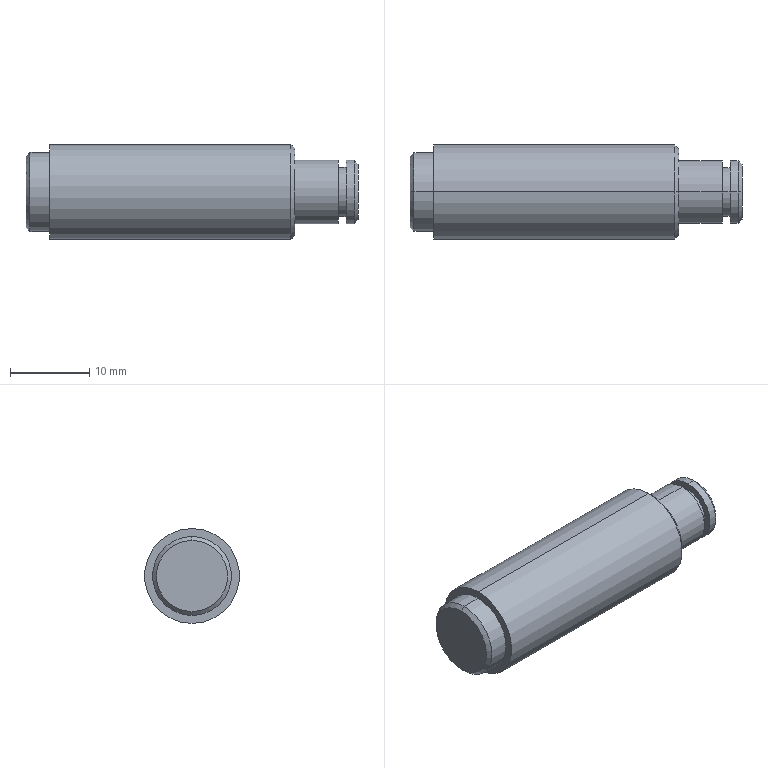Part | STEP file | 1 solid | 22 faces | box 42 x 12 x 12 mm | volume 4112 mm3 | cylinder 10 | cone 6 | plane 6 | commonest cylinder face diameters 8 x4 6.2 x2 10 x2 12 x2
STEP:
#1=CARTESIAN_POINT('',(0.,0.,0.));
#2=DIRECTION('',(0.,0.,1.));
#3=DIRECTION('',(1.,0.,0.));
#4=AXIS2_PLACEMENT_3D('',#1,#2,#3);
#5=CARTESIAN_POINT('',(3.,0.,-6.));
#6=VERTEX_POINT('',#5);
#7=CARTESIAN_POINT('',(3.,0.,6.));
#8=VERTEX_POINT('',#7);
#9=CARTESIAN_POINT('',(3.,0.,0.));
#10=DIRECTION('',(1.,0.,0.));
#11=DIRECTION('',(0.,0.,-1.));
#12=AXIS2_PLACEMENT_3D('',#9,#10,#11);
#13=CIRCLE('',#12,6.);
#14=CARTESIAN_POINT('',(18.5,0.,0.));
#15=DIRECTION('',(1.,0.,0.));
#16=DIRECTION('',(0.,0.,-1.));
#17=AXIS2_PLACEMENT_3D('',#14,#15,#16);
#18=CYLINDRICAL_SURFACE('',#17,6.);
#19=CARTESIAN_POINT('',(0.,-15.5));
#20=DIRECTION('',(1.,0.));
#21=VECTOR('',#20,1.);
#22=LINE('',#19,#21);
#23=(GEOMETRIC_REPRESENTATION_CONTEXT(2)PARAMETRIC_REPRESENTATION_CONTEXT()REPRESENTATION_CONTEXT('',''));
#24=DEFINITIONAL_REPRESENTATION('',(#22),#23);
#25=PCURVE('',#18,#24);
#26=CARTESIAN_POINT('',(3.,5.5,0.));
#27=DIRECTION('',(-1.,0.,0.));
#28=DIRECTION('',(0.,0.,1.));
#29=AXIS2_PLACEMENT_3D('',#26,#27,#28);
#30=PLANE('',#29);
#31=CARTESIAN_POINT('',(-6.,-5.5));
#32=CARTESIAN_POINT('',(-6.,4.892));
#33=CARTESIAN_POINT('',(3.,-0.3038));
#34=CARTESIAN_POINT('',(12.,-5.5));
#35=CARTESIAN_POINT('',(3.,-10.696));
#36=CARTESIAN_POINT('',(-6.,-15.892));
#37=CARTESIAN_POINT('',(-6.,-5.5));
#38=(BOUNDED_CURVE()B_SPLINE_CURVE(2,(#31,#32,#33,#34,#35,#36,#37),.UNSPECIFIED.,.T.,.F.)B_SPLINE_CURVE_WITH_KNOTS((1,2,2,2,2,1),(-2.094,0.,2.094,4.189,6.283,8.378),.UNSPECIFIED.)CURVE()GEOMETRIC_REPRESENTATION_ITEM()RATIONAL_B_SPLINE_CURVE((1.,0.5,1.,0.5,1.,0.5,1.))REPRESENTATION_ITEM(''));
#39=(GEOMETRIC_REPRESENTATION_CONTEXT(2)PARAMETRIC_REPRESENTATION_CONTEXT()REPRESENTATION_CONTEXT('',''));
#40=DEFINITIONAL_REPRESENTATION('',(#38),#39);
#41=PCURVE('',#30,#40);
#42=SURFACE_CURVE('',#13,(#25,#41),.PCURVE_S1.);
#43=EDGE_CURVE('',#6,#8,#42,.T.);
#44=ORIENTED_EDGE('',*,*,#43,.T.);
#45=CARTESIAN_POINT('',(33.5,0.,6.));
#46=VERTEX_POINT('',#45);
#47=CARTESIAN_POINT('',(18.5,0.,6.));
#48=DIRECTION('',(1.,0.,0.));
#49=VECTOR('',#48,1.);
#50=LINE('',#47,#49);
#51=CARTESIAN_POINT('',(3.142,0.));
#52=DIRECTION('',(0.,1.));
#53=VECTOR('',#52,1.);
#54=LINE('',#51,#53);
#55=(GEOMETRIC_REPRESENTATION_CONTEXT(2)PARAMETRIC_REPRESENTATION_CONTEXT()REPRESENTATION_CONTEXT('',''));
#56=DEFINITIONAL_REPRESENTATION('',(#54),#55);
#57=PCURVE('',#18,#56);
#58=CARTESIAN_POINT('',(18.5,0.,0.));
#59=DIRECTION('',(1.,0.,0.));
#60=DIRECTION('',(0.,0.,-1.));
#61=AXIS2_PLACEMENT_3D('',#58,#59,#60);
#62=CYLINDRICAL_SURFACE('',#61,6.);
#63=CARTESIAN_POINT('',(3.142,0.));
#64=DIRECTION('',(0.,1.));
#65=VECTOR('',#64,1.);
#66=LINE('',#63,#65);
#67=(GEOMETRIC_REPRESENTATION_CONTEXT(2)PARAMETRIC_REPRESENTATION_CONTEXT()REPRESENTATION_CONTEXT('',''));
#68=DEFINITIONAL_REPRESENTATION('',(#66),#67);
#69=PCURVE('',#62,#68);
#70=SURFACE_CURVE('',#50,(#57,#69),.PCURVE_S1.);
#71=EDGE_CURVE('',#8,#46,#70,.T.);
#72=ORIENTED_EDGE('',*,*,#71,.T.);
#73=CARTESIAN_POINT('',(33.5,0.,-6.));
#74=VERTEX_POINT('',#73);
#75=CARTESIAN_POINT('',(33.5,0.,0.));
#76=DIRECTION('',(-1.,0.,0.));
#77=DIRECTION('',(0.,0.,-1.));
#78=AXIS2_PLACEMENT_3D('',#75,#76,#77);
#79=CIRCLE('',#78,6.);
#80=CARTESIAN_POINT('',(6.283,15.));
#81=DIRECTION('',(-1.,0.));
#82=VECTOR('',#81,1.);
#83=LINE('',#80,#82);
#84=(GEOMETRIC_REPRESENTATION_CONTEXT(2)PARAMETRIC_REPRESENTATION_CONTEXT()REPRESENTATION_CONTEXT('',''));
#85=DEFINITIONAL_REPRESENTATION('',(#83),#84);
#86=PCURVE('',#18,#85);
#87=CARTESIAN_POINT('',(33.5,0.,0.));
#88=DIRECTION('',(-1.,0.,0.));
#89=DIRECTION('',(0.,0.,1.));
#90=AXIS2_PLACEMENT_3D('',#87,#88,#89);
#91=CONICAL_SURFACE('',#90,6.,0.7854);
#92=CARTESIAN_POINT('',(-3.142,0.));
#93=DIRECTION('',(1.,0.));
#94=VECTOR('',#93,1.);
#95=LINE('',#92,#94);
#96=(GEOMETRIC_REPRESENTATION_CONTEXT(2)PARAMETRIC_REPRESENTATION_CONTEXT()REPRESENTATION_CONTEXT('',''));
#97=DEFINITIONAL_REPRESENTATION('',(#95),#96);
#98=PCURVE('',#91,#97);
#99=SURFACE_CURVE('',#79,(#86,#98),.PCURVE_S1.);
#100=EDGE_CURVE('',#46,#74,#99,.T.);
#101=ORIENTED_EDGE('',*,*,#100,.T.);
#102=CARTESIAN_POINT('',(18.5,0.,-6.));
#103=DIRECTION('',(1.,0.,0.));
#104=VECTOR('',#103,1.);
#105=LINE('',#102,#104);
#106=CARTESIAN_POINT('',(0.,0.));
#107=DIRECTION('',(0.,1.));
#108=VECTOR('',#107,1.);
#109=LINE('',#106,#108);
#110=(GEOMETRIC_REPRESENTATION_CONTEXT(2)PARAMETRIC_REPRESENTATION_CONTEXT()REPRESENTATION_CONTEXT('',''));
#111=DEFINITIONAL_REPRESENTATION('',(#109),#110);
#112=PCURVE('',#18,#111);
#113=CARTESIAN_POINT('',(6.283,0.));
#114=DIRECTION('',(0.,1.));
#115=VECTOR('',#114,1.);
#116=LINE('',#113,#115);
#117=(GEOMETRIC_REPRESENTATION_CONTEXT(2)PARAMETRIC_REPRESENTATION_CONTEXT()REPRESENTATION_CONTEXT('',''));
#118=DEFINITIONAL_REPRESENTATION('',(#116),#117);
#119=PCURVE('',#62,#118);
#120=SURFACE_CURVE('',#105,(#112,#119),.PCURVE_S1.);
#121=EDGE_CURVE('',#6,#74,#120,.T.);
#122=ORIENTED_EDGE('',*,*,#121,.F.);
#123=EDGE_LOOP('',(#44,#72,#101,#122));
#124=FACE_BOUND('',#123,.T.);
#125=ADVANCED_FACE('',(#124),#18,.T.);
#126=CARTESIAN_POINT('',(34.,0.,5.5));
#127=VERTEX_POINT('',#126);
#128=CARTESIAN_POINT('',(34.,0.,-5.5));
#129=VERTEX_POINT('',#128);
#130=CARTESIAN_POINT('',(34.,0.,0.));
#131=DIRECTION('',(-1.,0.,0.));
#132=DIRECTION('',(0.,0.,1.));
#133=AXIS2_PLACEMENT_3D('',#130,#131,#132);
#134=CIRCLE('',#133,5.5);
#135=CARTESIAN_POINT('',(0.,-0.5));
#136=DIRECTION('',(1.,0.));
#137=VECTOR('',#136,1.);
#138=LINE('',#135,#137);
#139=(GEOMETRIC_REPRESENTATION_CONTEXT(2)PARAMETRIC_REPRESENTATION_CONTEXT()REPRESENTATION_CONTEXT('',''));
#140=DEFINITIONAL_REPRESENTATION('',(#138),#139);
#141=PCURVE('',#91,#140);
#142=CARTESIAN_POINT('',(34.,5.,0.));
#143=DIRECTION('',(1.,0.,0.));
#144=DIRECTION('',(0.,0.,-1.));
#145=AXIS2_PLACEMENT_3D('',#142,#143,#144);
#146=PLANE('',#145);
#147=CARTESIAN_POINT('',(-5.5,-5.));
#148=CARTESIAN_POINT('',(-5.5,4.526));
#149=CARTESIAN_POINT('',(2.75,-0.2369));
#150=CARTESIAN_POINT('',(11.,-5.));
#151=CARTESIAN_POINT('',(2.75,-9.763));
#152=CARTESIAN_POINT('',(-5.5,-14.526));
#153=CARTESIAN_POINT('',(-5.5,-5.));
#154=(BOUNDED_CURVE()B_SPLINE_CURVE(2,(#147,#148,#149,#150,#151,#152,#153),.UNSPECIFIED.,.T.,.F.)B_SPLINE_CURVE_WITH_KNOTS((1,2,2,2,2,1),(-2.094,0.,2.094,4.189,6.283,8.378),.UNSPECIFIED.)CURVE()GEOMETRIC_REPRESENTATION_ITEM()RATIONAL_B_SPLINE_CURVE((1.,0.5,1.,0.5,1.,0.5,1.))REPRESENTATION_ITEM(''));
#155=(GEOMETRIC_REPRESENTATION_CONTEXT(2)PARAMETRIC_REPRESENTATION_CONTEXT()REPRESENTATION_CONTEXT('',''));
#156=DEFINITIONAL_REPRESENTATION('',(#154),#155);
#157=PCURVE('',#146,#156);
#158=SURFACE_CURVE('',#134,(#141,#157),.PCURVE_S1.);
#159=EDGE_CURVE('',#127,#129,#158,.T.);
#160=ORIENTED_EDGE('',*,*,#159,.T.);
#161=CARTESIAN_POINT('',(33.5,0.,-6.));
#162=DIRECTION('',(-0.7071,0.,-0.7071));
#163=VECTOR('',#162,1.);
#164=LINE('',#161,#163);
#165=CARTESIAN_POINT('',(3.142,0.));
#166=DIRECTION('',(0.,1.));
#167=VECTOR('',#166,1.);
#168=LINE('',#165,#167);
#169=(GEOMETRIC_REPRESENTATION_CONTEXT(2)PARAMETRIC_REPRESENTATION_CONTEXT()REPRESENTATION_CONTEXT('',''));
#170=DEFINITIONAL_REPRESENTATION('',(#168),#169);
#171=PCURVE('',#91,#170);
#172=CARTESIAN_POINT('',(33.5,0.,0.));
#173=DIRECTION('',(-1.,0.,0.));
#174=DIRECTION('',(0.,0.,1.));
#175=AXIS2_PLACEMENT_3D('',#172,#173,#174);
#176=CONICAL_SURFACE('',#175,6.,0.7854);
#177=CARTESIAN_POINT('',(3.142,0.));
#178=DIRECTION('',(0.,1.));
#179=VECTOR('',#178,1.);
#180=LINE('',#177,#179);
#181=(GEOMETRIC_REPRESENTATION_CONTEXT(2)PARAMETRIC_REPRESENTATION_CONTEXT()REPRESENTATION_CONTEXT('',''));
#182=DEFINITIONAL_REPRESENTATION('',(#180),#181);
#183=PCURVE('',#176,#182);
#184=SURFACE_CURVE('',#164,(#171,#183),.PCURVE_S1.);
#185=EDGE_CURVE('',#129,#74,#184,.T.);
#186=ORIENTED_EDGE('',*,*,#185,.T.);
#187=ORIENTED_EDGE('',*,*,#100,.F.);
#188=CARTESIAN_POINT('',(33.5,0.,6.));
#189=DIRECTION('',(-0.7071,0.,0.7071));
#190=VECTOR('',#189,1.);
#191=LINE('',#188,#190);
#192=CARTESIAN_POINT('',(0.,0.));
#193=DIRECTION('',(0.,1.));
#194=VECTOR('',#193,1.);
#195=LINE('',#192,#194);
#196=(GEOMETRIC_REPRESENTATION_CONTEXT(2)PARAMETRIC_REPRESENTATION_CONTEXT()REPRESENTATION_CONTEXT('',''));
#197=DEFINITIONAL_REPRESENTATION('',(#195),#196);
#198=PCURVE('',#91,#197);
#199=CARTESIAN_POINT('',(6.283,0.));
#200=DIRECTION('',(0.,1.));
#201=VECTOR('',#200,1.);
#202=LINE('',#199,#201);
#203=(GEOMETRIC_REPRESENTATION_CONTEXT(2)PARAMETRIC_REPRESENTATION_CONTEXT()REPRESENTATION_CONTEXT('',''));
#204=DEFINITIONAL_REPRESENTATION('',(#202),#203);
#205=PCURVE('',#176,#204);
#206=SURFACE_CURVE('',#191,(#198,#205),.PCURVE_S1.);
#207=EDGE_CURVE('',#127,#46,#206,.T.);
#208=ORIENTED_EDGE('',*,*,#207,.F.);
#209=EDGE_LOOP('',(#160,#186,#187,#208));
#210=FACE_BOUND('',#209,.T.);
#211=ADVANCED_FACE('',(#210),#91,.T.);
#212=CARTESIAN_POINT('',(0.5,0.,-5.));
#213=VERTEX_POINT('',#212);
#214=CARTESIAN_POINT('',(0.5,0.,5.));
#215=VERTEX_POINT('',#214);
#216=CARTESIAN_POINT('',(0.5,0.,0.));
#217=DIRECTION('',(1.,0.,0.));
#218=DIRECTION('',(0.,0.,-1.));
#219=AXIS2_PLACEMENT_3D('',#216,#217,#218);
#220=CIRCLE('',#219,5.);
#221=CARTESIAN_POINT('',(1.5,0.,0.));
#222=DIRECTION('',(1.,0.,0.));
#223=DIRECTION('',(0.,0.,-1.));
#224=AXIS2_PLACEMENT_3D('',#221,#222,#223);
#225=CYLINDRICAL_SURFACE('',#224,5.);
#226=CARTESIAN_POINT('',(0.,-1.));
#227=DIRECTION('',(1.,0.));
#228=VECTOR('',#227,1.);
#229=LINE('',#226,#228);
#230=(GEOMETRIC_REPRESENTATION_CONTEXT(2)PARAMETRIC_REPRESENTATION_CONTEXT()REPRESENTATION_CONTEXT('',''));
#231=DEFINITIONAL_REPRESENTATION('',(#229),#230);
#232=PCURVE('',#225,#231);
#233=CARTESIAN_POINT('',(0.5,0.,0.));
#234=DIRECTION('',(1.,0.,0.));
#235=DIRECTION('',(0.,0.,-1.));
#236=AXIS2_PLACEMENT_3D('',#233,#234,#235);
#237=CONICAL_SURFACE('',#236,5.,0.7854);
#238=CARTESIAN_POINT('',(0.,0.));
#239=DIRECTION('',(1.,0.));
#240=VECTOR('',#239,1.);
#241=LINE('',#238,#240);
#242=(GEOMETRIC_REPRESENTATION_CONTEXT(2)PARAMETRIC_REPRESENTATION_CONTEXT()REPRESENTATION_CONTEXT('',''));
#243=DEFINITIONAL_REPRESENTATION('',(#241),#242);
#244=PCURVE('',#237,#243);
#245=SURFACE_CURVE('',#220,(#232,#244),.PCURVE_S1.);
#246=EDGE_CURVE('',#213,#215,#245,.T.);
#247=ORIENTED_EDGE('',*,*,#246,.T.);
#248=CARTESIAN_POINT('',(3.,0.,5.));
#249=VERTEX_POINT('',#248);
#250=CARTESIAN_POINT('',(1.5,0.,5.));
#251=DIRECTION('',(1.,0.,0.));
#252=VECTOR('',#251,1.);
#253=LINE('',#250,#252);
#254=CARTESIAN_POINT('',(3.142,0.));
#255=DIRECTION('',(0.,1.));
#256=VECTOR('',#255,1.);
#257=LINE('',#254,#256);
#258=(GEOMETRIC_REPRESENTATION_CONTEXT(2)PARAMETRIC_REPRESENTATION_CONTEXT()REPRESENTATION_CONTEXT('',''));
#259=DEFINITIONAL_REPRESENTATION('',(#257),#258);
#260=PCURVE('',#225,#259);
#261=CARTESIAN_POINT('',(1.5,0.,0.));
#262=DIRECTION('',(1.,0.,0.));
#263=DIRECTION('',(0.,0.,-1.));
#264=AXIS2_PLACEMENT_3D('',#261,#262,#263);
#265=CYLINDRICAL_SURFACE('',#264,5.);
#266=CARTESIAN_POINT('',(3.142,0.));
#267=DIRECTION('',(0.,1.));
#268=VECTOR('',#267,1.);
#269=LINE('',#266,#268);
#270=(GEOMETRIC_REPRESENTATION_CONTEXT(2)PARAMETRIC_REPRESENTATION_CONTEXT()REPRESENTATION_CONTEXT('',''));
#271=DEFINITIONAL_REPRESENTATION('',(#269),#270);
#272=PCURVE('',#265,#271);
#273=SURFACE_CURVE('',#253,(#260,#272),.PCURVE_S1.);
#274=EDGE_CURVE('',#215,#249,#273,.T.);
#275=ORIENTED_EDGE('',*,*,#274,.T.);
#276=CARTESIAN_POINT('',(3.,0.,-5.));
#277=VERTEX_POINT('',#276);
#278=CARTESIAN_POINT('',(3.,0.,0.));
#279=DIRECTION('',(1.,0.,0.));
#280=DIRECTION('',(0.,0.,-1.));
#281=AXIS2_PLACEMENT_3D('',#278,#279,#280);
#282=CIRCLE('',#281,5.);
#283=CARTESIAN_POINT('',(0.,1.5));
#284=DIRECTION('',(1.,0.));
#285=VECTOR('',#284,1.);
#286=LINE('',#283,#285);
#287=(GEOMETRIC_REPRESENTATION_CONTEXT(2)PARAMETRIC_REPRESENTATION_CONTEXT()REPRESENTATION_CONTEXT('',''));
#288=DEFINITIONAL_REPRESENTATION('',(#286),#287);
#289=PCURVE('',#225,#288);
#290=CARTESIAN_POINT('',(-5.,-5.5));
#291=CARTESIAN_POINT('',(-5.,3.16));
#292=CARTESIAN_POINT('',(2.5,-1.17));
#293=CARTESIAN_POINT('',(10.,-5.5));
#294=CARTESIAN_POINT('',(2.5,-9.83));
#295=CARTESIAN_POINT('',(-5.,-14.16));
#296=CARTESIAN_POINT('',(-5.,-5.5));
#297=(BOUNDED_CURVE()B_SPLINE_CURVE(2,(#290,#291,#292,#293,#294,#295,#296),.UNSPECIFIED.,.T.,.F.)B_SPLINE_CURVE_WITH_KNOTS((1,2,2,2,2,1),(-2.094,0.,2.094,4.189,6.283,8.378),.UNSPECIFIED.)CURVE()GEOMETRIC_REPRESENTATION_ITEM()RATIONAL_B_SPLINE_CURVE((1.,0.5,1.,0.5,1.,0.5,1.))REPRESENTATION_ITEM(''));
#298=(GEOMETRIC_REPRESENTATION_CONTEXT(2)PARAMETRIC_REPRESENTATION_CONTEXT()REPRESENTATION_CONTEXT('',''));
#299=DEFINITIONAL_REPRESENTATION('',(#297),#298);
#300=PCURVE('',#30,#299);
#301=SURFACE_CURVE('',#282,(#289,#300),.PCURVE_S1.);
#302=EDGE_CURVE('',#277,#249,#301,.T.);
#303=ORIENTED_EDGE('',*,*,#302,.F.);
#304=CARTESIAN_POINT('',(1.5,0.,-5.));
#305=DIRECTION('',(1.,0.,0.));
#306=VECTOR('',#305,1.);
#307=LINE('',#304,#306);
#308=CARTESIAN_POINT('',(0.,0.));
#309=DIRECTION('',(0.,1.));
#310=VECTOR('',#309,1.);
#311=LINE('',#308,#310);
#312=(GEOMETRIC_REPRESENTATION_CONTEXT(2)PARAMETRIC_REPRESENTATION_CONTEXT()REPRESENTATION_CONTEXT('',''));
#313=DEFINITIONAL_REPRESENTATION('',(#311),#312);
#314=PCURVE('',#225,#313);
#315=CARTESIAN_POINT('',(6.283,0.));
#316=DIRECTION('',(0.,1.));
#317=VECTOR('',#316,1.);
#318=LINE('',#315,#317);
#319=(GEOMETRIC_REPRESENTATION_CONTEXT(2)PARAMETRIC_REPRESENTATION_CONTEXT()REPRESENTATION_CONTEXT('',''));
#320=DEFINITIONAL_REPRESENTATION('',(#318),#319);
#321=PCURVE('',#265,#320);
#322=SURFACE_CURVE('',#307,(#314,#321),.PCURVE_S1.);
#323=EDGE_CURVE('',#213,#277,#322,.T.);
#324=ORIENTED_EDGE('',*,*,#323,.F.);
#325=EDGE_LOOP('',(#247,#275,#303,#324));
#326=FACE_BOUND('',#325,.T.);
#327=ADVANCED_FACE('',(#326),#225,.T.);
#328=CARTESIAN_POINT('',(34.,0.,4.));
#329=VERTEX_POINT('',#328);
#330=CARTESIAN_POINT('',(34.,0.,-4.));
#331=VERTEX_POINT('',#330);
#332=CARTESIAN_POINT('',(34.,0.,0.));
#333=DIRECTION('',(-1.,0.,0.));
#334=DIRECTION('',(0.,0.,-1.));
#335=AXIS2_PLACEMENT_3D('',#332,#333,#334);
#336=CIRCLE('',#335,4.);
#337=CARTESIAN_POINT('',(36.75,0.,0.));
#338=DIRECTION('',(1.,0.,0.));
#339=DIRECTION('',(0.,0.,-1.));
#340=AXIS2_PLACEMENT_3D('',#337,#338,#339);
#341=CYLINDRICAL_SURFACE('',#340,4.);
#342=CARTESIAN_POINT('',(6.283,-2.75));
#343=DIRECTION('',(-1.,0.));
#344=VECTOR('',#343,1.);
#345=LINE('',#342,#344);
#346=(GEOMETRIC_REPRESENTATION_CONTEXT(2)PARAMETRIC_REPRESENTATION_CONTEXT()REPRESENTATION_CONTEXT('',''));
#347=DEFINITIONAL_REPRESENTATION('',(#345),#346);
#348=PCURVE('',#341,#347);
#349=CARTESIAN_POINT('',(4.,-5.));
#350=CARTESIAN_POINT('',(4.,-11.928));
#351=CARTESIAN_POINT('',(-2.,-8.464));
#352=CARTESIAN_POINT('',(-8.,-5.));
#353=CARTESIAN_POINT('',(-2.,-1.536));
#354=CARTESIAN_POINT('',(4.,1.928));
#355=CARTESIAN_POINT('',(4.,-5.));
#356=(BOUNDED_CURVE()B_SPLINE_CURVE(2,(#349,#350,#351,#352,#353,#354,#355),.UNSPECIFIED.,.T.,.F.)B_SPLINE_CURVE_WITH_KNOTS((1,2,2,2,2,1),(-2.094,0.,2.094,4.189,6.283,8.378),.UNSPECIFIED.)CURVE()GEOMETRIC_REPRESENTATION_ITEM()RATIONAL_B_SPLINE_CURVE((1.,0.5,1.,0.5,1.,0.5,1.))REPRESENTATION_ITEM(''));
#357=(GEOMETRIC_REPRESENTATION_CONTEXT(2)PARAMETRIC_REPRESENTATION_CONTEXT()REPRESENTATION_CONTEXT('',''));
#358=DEFINITIONAL_REPRESENTATION('',(#356),#357);
#359=PCURVE('',#146,#358);
#360=SURFACE_CURVE('',#336,(#348,#359),.PCURVE_S1.);
#361=EDGE_CURVE('',#329,#331,#360,.T.);
#362=ORIENTED_EDGE('',*,*,#361,.F.);
#363=CARTESIAN_POINT('',(39.5,0.,4.));
#364=VERTEX_POINT('',#363);
#365=CARTESIAN_POINT('',(36.75,0.,4.));
#366=DIRECTION('',(1.,0.,0.));
#367=VECTOR('',#366,1.);
#368=LINE('',#365,#367);
#369=CARTESIAN_POINT('',(3.142,0.));
#370=DIRECTION('',(0.,1.));
#371=VECTOR('',#370,1.);
#372=LINE('',#369,#371);
#373=(GEOMETRIC_REPRESENTATION_CONTEXT(2)PARAMETRIC_REPRESENTATION_CONTEXT()REPRESENTATION_CONTEXT('',''));
#374=DEFINITIONAL_REPRESENTATION('',(#372),#373);
#375=PCURVE('',#341,#374);
#376=CARTESIAN_POINT('',(36.75,0.,0.));
#377=DIRECTION('',(1.,0.,0.));
#378=DIRECTION('',(0.,0.,-1.));
#379=AXIS2_PLACEMENT_3D('',#376,#377,#378);
#380=CYLINDRICAL_SURFACE('',#379,4.);
#381=CARTESIAN_POINT('',(3.142,0.));
#382=DIRECTION('',(0.,1.));
#383=VECTOR('',#382,1.);
#384=LINE('',#381,#383);
#385=(GEOMETRIC_REPRESENTATION_CONTEXT(2)PARAMETRIC_REPRESENTATION_CONTEXT()REPRESENTATION_CONTEXT('',''));
#386=DEFINITIONAL_REPRESENTATION('',(#384),#385);
#387=PCURVE('',#380,#386);
#388=SURFACE_CURVE('',#368,(#375,#387),.PCURVE_S1.);
#389=EDGE_CURVE('',#329,#364,#388,.T.);
#390=ORIENTED_EDGE('',*,*,#389,.T.);
#391=CARTESIAN_POINT('',(39.5,0.,-4.));
#392=VERTEX_POINT('',#391);
#393=CARTESIAN_POINT('',(39.5,0.,0.));
#394=DIRECTION('',(-1.,0.,0.));
#395=DIRECTION('',(0.,0.,-1.));
#396=AXIS2_PLACEMENT_3D('',#393,#394,#395);
#397=CIRCLE('',#396,4.);
#398=CARTESIAN_POINT('',(6.283,2.75));
#399=DIRECTION('',(-1.,0.));
#400=VECTOR('',#399,1.);
#401=LINE('',#398,#400);
#402=(GEOMETRIC_REPRESENTATION_CONTEXT(2)PARAMETRIC_REPRESENTATION_CONTEXT()REPRESENTATION_CONTEXT('',''));
#403=DEFINITIONAL_REPRESENTATION('',(#401),#402);
#404=PCURVE('',#341,#403);
#405=CARTESIAN_POINT('',(39.5,3.55,0.));
#406=DIRECTION('',(1.,0.,0.));
#407=DIRECTION('',(0.,0.,-1.));
#408=AXIS2_PLACEMENT_3D('',#405,#406,#407);
#409=PLANE('',#408);
#410=CARTESIAN_POINT('',(4.,-3.55));
#411=CARTESIAN_POINT('',(4.,-10.478));
#412=CARTESIAN_POINT('',(-2.,-7.014));
#413=CARTESIAN_POINT('',(-8.,-3.55));
#414=CARTESIAN_POINT('',(-2.,-0.0859));
#415=CARTESIAN_POINT('',(4.,3.378));
#416=CARTESIAN_POINT('',(4.,-3.55));
#417=(BOUNDED_CURVE()B_SPLINE_CURVE(2,(#410,#411,#412,#413,#414,#415,#416),.UNSPECIFIED.,.T.,.F.)B_SPLINE_CURVE_WITH_KNOTS((1,2,2,2,2,1),(-2.094,0.,2.094,4.189,6.283,8.378),.UNSPECIFIED.)CURVE()GEOMETRIC_REPRESENTATION_ITEM()RATIONAL_B_SPLINE_CURVE((1.,0.5,1.,0.5,1.,0.5,1.))REPRESENTATION_ITEM(''));
#418=(GEOMETRIC_REPRESENTATION_CONTEXT(2)PARAMETRIC_REPRESENTATION_CONTEXT()REPRESENTATION_CONTEXT('',''));
#419=DEFINITIONAL_REPRESENTATION('',(#417),#418);
#420=PCURVE('',#409,#419);
#421=SURFACE_CURVE('',#397,(#404,#420),.PCURVE_S1.);
#422=EDGE_CURVE('',#364,#392,#421,.T.);
#423=ORIENTED_EDGE('',*,*,#422,.T.);
#424=CARTESIAN_POINT('',(36.75,0.,-4.));
#425=DIRECTION('',(1.,0.,0.));
#426=VECTOR('',#425,1.);
#427=LINE('',#424,#426);
#428=CARTESIAN_POINT('',(0.,0.));
#429=DIRECTION('',(0.,1.));
#430=VECTOR('',#429,1.);
#431=LINE('',#428,#430);
#432=(GEOMETRIC_REPRESENTATION_CONTEXT(2)PARAMETRIC_REPRESENTATION_CONTEXT()REPRESENTATION_CONTEXT('',''));
#433=DEFINITIONAL_REPRESENTATION('',(#431),#432);
#434=PCURVE('',#341,#433);
#435=CARTESIAN_POINT('',(6.283,0.));
#436=DIRECTION('',(0.,1.));
#437=VECTOR('',#436,1.);
#438=LINE('',#435,#437);
#439=(GEOMETRIC_REPRESENTATION_CONTEXT(2)PARAMETRIC_REPRESENTATION_CONTEXT()REPRESENTATION_CONTEXT('',''));
#440=DEFINITIONAL_REPRESENTATION('',(#438),#439);
#441=PCURVE('',#380,#440);
#442=SURFACE_CURVE('',#427,(#434,#441),.PCURVE_S1.);
#443=EDGE_CURVE('',#331,#392,#442,.T.);
#444=ORIENTED_EDGE('',*,*,#443,.F.);
#445=EDGE_LOOP('',(#362,#390,#423,#444));
#446=FACE_BOUND('',#445,.T.);
#447=ADVANCED_FACE('',(#446),#341,.T.);
#448=CARTESIAN_POINT('',(0.,0.,-4.5));
#449=VERTEX_POINT('',#448);
#450=CARTESIAN_POINT('',(0.,0.,4.5));
#451=VERTEX_POINT('',#450);
#452=CARTESIAN_POINT('',(0.,0.,0.));
#453=DIRECTION('',(1.,0.,0.));
#454=DIRECTION('',(0.,0.,-1.));
#455=AXIS2_PLACEMENT_3D('',#452,#453,#454);
#456=CIRCLE('',#455,4.5);
#457=CARTESIAN_POINT('',(0.,-0.5));
#458=DIRECTION('',(1.,0.));
#459=VECTOR('',#458,1.);
#460=LINE('',#457,#459);
#461=(GEOMETRIC_REPRESENTATION_CONTEXT(2)PARAMETRIC_REPRESENTATION_CONTEXT()REPRESENTATION_CONTEXT('',''));
#462=DEFINITIONAL_REPRESENTATION('',(#460),#461);
#463=PCURVE('',#237,#462);
#464=CARTESIAN_POINT('',(0.,2.5,0.));
#465=DIRECTION('',(-1.,0.,0.));
#466=DIRECTION('',(0.,0.,1.));
#467=AXIS2_PLACEMENT_3D('',#464,#465,#466);
#468=PLANE('',#467);
#469=CARTESIAN_POINT('',(-4.5,-2.5));
#470=CARTESIAN_POINT('',(-4.5,5.294));
#471=CARTESIAN_POINT('',(2.25,1.397));
#472=CARTESIAN_POINT('',(9.,-2.5));
#473=CARTESIAN_POINT('',(2.25,-6.397));
#474=CARTESIAN_POINT('',(-4.5,-10.294));
#475=CARTESIAN_POINT('',(-4.5,-2.5));
#476=(BOUNDED_CURVE()B_SPLINE_CURVE(2,(#469,#470,#471,#472,#473,#474,#475),.UNSPECIFIED.,.T.,.F.)B_SPLINE_CURVE_WITH_KNOTS((1,2,2,2,2,1),(-2.094,0.,2.094,4.189,6.283,8.378),.UNSPECIFIED.)CURVE()GEOMETRIC_REPRESENTATION_ITEM()RATIONAL_B_SPLINE_CURVE((1.,0.5,1.,0.5,1.,0.5,1.))REPRESENTATION_ITEM(''));
#477=(GEOMETRIC_REPRESENTATION_CONTEXT(2)PARAMETRIC_REPRESENTATION_CONTEXT()REPRESENTATION_CONTEXT('',''));
#478=DEFINITIONAL_REPRESENTATION('',(#476),#477);
#479=PCURVE('',#468,#478);
#480=SURFACE_CURVE('',#456,(#463,#479),.PCURVE_S1.);
#481=EDGE_CURVE('',#449,#451,#480,.T.);
#482=ORIENTED_EDGE('',*,*,#481,.T.);
#483=CARTESIAN_POINT('',(0.5,0.,5.));
#484=DIRECTION('',(0.7071,0.,0.7071));
#485=VECTOR('',#484,1.);
#486=LINE('',#483,#485);
#487=CARTESIAN_POINT('',(3.142,0.));
#488=DIRECTION('',(0.,1.));
#489=VECTOR('',#488,1.);
#490=LINE('',#487,#489);
#491=(GEOMETRIC_REPRESENTATION_CONTEXT(2)PARAMETRIC_REPRESENTATION_CONTEXT()REPRESENTATION_CONTEXT('',''));
#492=DEFINITIONAL_REPRESENTATION('',(#490),#491);
#493=PCURVE('',#237,#492);
#494=CARTESIAN_POINT('',(0.5,0.,0.));
#495=DIRECTION('',(1.,0.,0.));
#496=DIRECTION('',(0.,0.,-1.));
#497=AXIS2_PLACEMENT_3D('',#494,#495,#496);
#498=CONICAL_SURFACE('',#497,5.,0.7854);
#499=CARTESIAN_POINT('',(3.142,0.));
#500=DIRECTION('',(0.,1.));
#501=VECTOR('',#500,1.);
#502=LINE('',#499,#501);
#503=(GEOMETRIC_REPRESENTATION_CONTEXT(2)PARAMETRIC_REPRESENTATION_CONTEXT()REPRESENTATION_CONTEXT('',''));
#504=DEFINITIONAL_REPRESENTATION('',(#502),#503);
#505=PCURVE('',#498,#504);
#506=SURFACE_CURVE('',#486,(#493,#505),.PCURVE_S1.);
#507=EDGE_CURVE('',#451,#215,#506,.T.);
#508=ORIENTED_EDGE('',*,*,#507,.T.);
#509=ORIENTED_EDGE('',*,*,#246,.F.);
#510=CARTESIAN_POINT('',(0.5,0.,-5.));
#511=DIRECTION('',(0.7071,0.,-0.7071));
#512=VECTOR('',#511,1.);
#513=LINE('',#510,#512);
#514=CARTESIAN_POINT('',(0.,0.));
#515=DIRECTION('',(0.,1.));
#516=VECTOR('',#515,1.);
#517=LINE('',#514,#516);
#518=(GEOMETRIC_REPRESENTATION_CONTEXT(2)PARAMETRIC_REPRESENTATION_CONTEXT()REPRESENTATION_CONTEXT('',''));
#519=DEFINITIONAL_REPRESENTATION('',(#517),#518);
#520=PCURVE('',#237,#519);
#521=CARTESIAN_POINT('',(6.283,0.));
#522=DIRECTION('',(0.,1.));
#523=VECTOR('',#522,1.);
#524=LINE('',#521,#523);
#525=(GEOMETRIC_REPRESENTATION_CONTEXT(2)PARAMETRIC_REPRESENTATION_CONTEXT()REPRESENTATION_CONTEXT('',''));
#526=DEFINITIONAL_REPRESENTATION('',(#524),#525);
#527=PCURVE('',#498,#526);
#528=SURFACE_CURVE('',#513,(#520,#527),.PCURVE_S1.);
#529=EDGE_CURVE('',#449,#213,#528,.T.);
#530=ORIENTED_EDGE('',*,*,#529,.F.);
#531=EDGE_LOOP('',(#482,#508,#509,#530));
#532=FACE_BOUND('',#531,.T.);
#533=ADVANCED_FACE('',(#532),#237,.T.);
#534=CARTESIAN_POINT('',(39.5,0.,3.1));
#535=VERTEX_POINT('',#534);
#536=CARTESIAN_POINT('',(39.5,0.,-3.1));
#537=VERTEX_POINT('',#536);
#538=CARTESIAN_POINT('',(39.5,0.,0.));
#539=DIRECTION('',(-1.,0.,0.));
#540=DIRECTION('',(0.,0.,-1.));
#541=AXIS2_PLACEMENT_3D('',#538,#539,#540);
#542=CIRCLE('',#541,3.1);
#543=CARTESIAN_POINT('',(40.,0.,0.));
#544=DIRECTION('',(1.,0.,0.));
#545=DIRECTION('',(0.,0.,-1.));
#546=AXIS2_PLACEMENT_3D('',#543,#544,#545);
#547=CYLINDRICAL_SURFACE('',#546,3.1);
#548=CARTESIAN_POINT('',(6.283,-0.5));
#549=DIRECTION('',(-1.,0.));
#550=VECTOR('',#549,1.);
#551=LINE('',#548,#550);
#552=(GEOMETRIC_REPRESENTATION_CONTEXT(2)PARAMETRIC_REPRESENTATION_CONTEXT()REPRESENTATION_CONTEXT('',''));
#553=DEFINITIONAL_REPRESENTATION('',(#551),#552);
#554=PCURVE('',#547,#553);
#555=CARTESIAN_POINT('',(3.1,-3.55));
#556=CARTESIAN_POINT('',(3.1,-8.919));
#557=CARTESIAN_POINT('',(-1.55,-6.235));
#558=CARTESIAN_POINT('',(-6.2,-3.55));
#559=CARTESIAN_POINT('',(-1.55,-0.8653));
#560=CARTESIAN_POINT('',(3.1,1.819));
#561=CARTESIAN_POINT('',(3.1,-3.55));
#562=(BOUNDED_CURVE()B_SPLINE_CURVE(2,(#555,#556,#557,#558,#559,#560,#561),.UNSPECIFIED.,.T.,.F.)B_SPLINE_CURVE_WITH_KNOTS((1,2,2,2,2,1),(-2.094,0.,2.094,4.189,6.283,8.378),.UNSPECIFIED.)CURVE()GEOMETRIC_REPRESENTATION_ITEM()RATIONAL_B_SPLINE_CURVE((1.,0.5,1.,0.5,1.,0.5,1.))REPRESENTATION_ITEM(''));
#563=(GEOMETRIC_REPRESENTATION_CONTEXT(2)PARAMETRIC_REPRESENTATION_CONTEXT()REPRESENTATION_CONTEXT('',''));
#564=DEFINITIONAL_REPRESENTATION('',(#562),#563);
#565=PCURVE('',#409,#564);
#566=SURFACE_CURVE('',#542,(#554,#565),.PCURVE_S1.);
#567=EDGE_CURVE('',#535,#537,#566,.T.);
#568=ORIENTED_EDGE('',*,*,#567,.F.);
#569=CARTESIAN_POINT('',(40.5,0.,3.1));
#570=VERTEX_POINT('',#569);
#571=CARTESIAN_POINT('',(40.,0.,3.1));
#572=DIRECTION('',(1.,0.,0.));
#573=VECTOR('',#572,1.);
#574=LINE('',#571,#573);
#575=CARTESIAN_POINT('',(3.142,0.));
#576=DIRECTION('',(0.,1.));
#577=VECTOR('',#576,1.);
#578=LINE('',#575,#577);
#579=(GEOMETRIC_REPRESENTATION_CONTEXT(2)PARAMETRIC_REPRESENTATION_CONTEXT()REPRESENTATION_CONTEXT('',''));
#580=DEFINITIONAL_REPRESENTATION('',(#578),#579);
#581=PCURVE('',#547,#580);
#582=CARTESIAN_POINT('',(40.,0.,0.));
#583=DIRECTION('',(1.,0.,0.));
#584=DIRECTION('',(0.,0.,-1.));
#585=AXIS2_PLACEMENT_3D('',#582,#583,#584);
#586=CYLINDRICAL_SURFACE('',#585,3.1);
#587=CARTESIAN_POINT('',(3.142,0.));
#588=DIRECTION('',(0.,1.));
#589=VECTOR('',#588,1.);
#590=LINE('',#587,#589);
#591=(GEOMETRIC_REPRESENTATION_CONTEXT(2)PARAMETRIC_REPRESENTATION_CONTEXT()REPRESENTATION_CONTEXT('',''));
#592=DEFINITIONAL_REPRESENTATION('',(#590),#591);
#593=PCURVE('',#586,#592);
#594=SURFACE_CURVE('',#574,(#581,#593),.PCURVE_S1.);
#595=EDGE_CURVE('',#535,#570,#594,.T.);
#596=ORIENTED_EDGE('',*,*,#595,.T.);
#597=CARTESIAN_POINT('',(40.5,0.,-3.1));
#598=VERTEX_POINT('',#597);
#599=CARTESIAN_POINT('',(40.5,0.,0.));
#600=DIRECTION('',(-1.,0.,0.));
#601=DIRECTION('',(0.,0.,-1.));
#602=AXIS2_PLACEMENT_3D('',#599,#600,#601);
#603=CIRCLE('',#602,3.1);
#604=CARTESIAN_POINT('',(6.283,0.5));
#605=DIRECTION('',(-1.,0.));
#606=VECTOR('',#605,1.);
#607=LINE('',#604,#606);
#608=(GEOMETRIC_REPRESENTATION_CONTEXT(2)PARAMETRIC_REPRESENTATION_CONTEXT()REPRESENTATION_CONTEXT('',''));
#609=DEFINITIONAL_REPRESENTATION('',(#607),#608);
#610=PCURVE('',#547,#609);
#611=CARTESIAN_POINT('',(40.5,3.55,0.));
#612=DIRECTION('',(-1.,0.,0.));
#613=DIRECTION('',(0.,0.,1.));
#614=AXIS2_PLACEMENT_3D('',#611,#612,#613);
#615=PLANE('',#614);
#616=CARTESIAN_POINT('',(0.,-3.55));
#617=DIRECTION('',(-1.,0.));
#618=AXIS2_PLACEMENT_2D('',#616,#617);
#619=CIRCLE('',#618,3.1);
#620=(GEOMETRIC_REPRESENTATION_CONTEXT(2)PARAMETRIC_REPRESENTATION_CONTEXT()REPRESENTATION_CONTEXT('',''));
#621=DEFINITIONAL_REPRESENTATION('',(#619),#620);
#622=PCURVE('',#615,#621);
#623=SURFACE_CURVE('',#603,(#610,#622),.PCURVE_S1.);
#624=EDGE_CURVE('',#570,#598,#623,.T.);
#625=ORIENTED_EDGE('',*,*,#624,.T.);
#626=CARTESIAN_POINT('',(40.,0.,-3.1));
#627=DIRECTION('',(1.,0.,0.));
#628=VECTOR('',#627,1.);
#629=LINE('',#626,#628);
#630=CARTESIAN_POINT('',(0.,0.));
#631=DIRECTION('',(0.,1.));
#632=VECTOR('',#631,1.);
#633=LINE('',#630,#632);
#634=(GEOMETRIC_REPRESENTATION_CONTEXT(2)PARAMETRIC_REPRESENTATION_CONTEXT()REPRESENTATION_CONTEXT('',''));
#635=DEFINITIONAL_REPRESENTATION('',(#633),#634);
#636=PCURVE('',#547,#635);
#637=CARTESIAN_POINT('',(6.283,0.));
#638=DIRECTION('',(0.,1.));
#639=VECTOR('',#638,1.);
#640=LINE('',#637,#639);
#641=(GEOMETRIC_REPRESENTATION_CONTEXT(2)PARAMETRIC_REPRESENTATION_CONTEXT()REPRESENTATION_CONTEXT('',''));
#642=DEFINITIONAL_REPRESENTATION('',(#640),#641);
#643=PCURVE('',#586,#642);
#644=SURFACE_CURVE('',#629,(#636,#643),.PCURVE_S1.);
#645=EDGE_CURVE('',#537,#598,#644,.T.);
#646=ORIENTED_EDGE('',*,*,#645,.F.);
#647=EDGE_LOOP('',(#568,#596,#625,#646));
#648=FACE_BOUND('',#647,.T.);
#649=ADVANCED_FACE('',(#648),#547,.T.);
#650=CARTESIAN_POINT('',(40.5,0.,4.));
#651=VERTEX_POINT('',#650);
#652=CARTESIAN_POINT('',(40.5,0.,-4.));
#653=VERTEX_POINT('',#652);
#654=CARTESIAN_POINT('',(40.5,0.,0.));
#655=DIRECTION('',(-1.,0.,0.));
#656=DIRECTION('',(0.,0.,-1.));
#657=AXIS2_PLACEMENT_3D('',#654,#655,#656);
#658=CIRCLE('',#657,4.);
#659=CARTESIAN_POINT('',(41.25,0.,0.));
#660=DIRECTION('',(1.,0.,0.));
#661=DIRECTION('',(0.,0.,-1.));
#662=AXIS2_PLACEMENT_3D('',#659,#660,#661);
#663=CYLINDRICAL_SURFACE('',#662,4.);
#664=CARTESIAN_POINT('',(6.283,-0.75));
#665=DIRECTION('',(-1.,0.));
#666=VECTOR('',#665,1.);
#667=LINE('',#664,#666);
#668=(GEOMETRIC_REPRESENTATION_CONTEXT(2)PARAMETRIC_REPRESENTATION_CONTEXT()REPRESENTATION_CONTEXT('',''));
#669=DEFINITIONAL_REPRESENTATION('',(#667),#668);
#670=PCURVE('',#663,#669);
#671=CARTESIAN_POINT('',(0.,-3.55));
#672=DIRECTION('',(-1.,0.));
#673=AXIS2_PLACEMENT_2D('',#671,#672);
#674=CIRCLE('',#673,4.);
#675=(GEOMETRIC_REPRESENTATION_CONTEXT(2)PARAMETRIC_REPRESENTATION_CONTEXT()REPRESENTATION_CONTEXT('',''));
#676=DEFINITIONAL_REPRESENTATION('',(#674),#675);
#677=PCURVE('',#615,#676);
#678=SURFACE_CURVE('',#658,(#670,#677),.PCURVE_S1.);
#679=EDGE_CURVE('',#651,#653,#678,.T.);
#680=ORIENTED_EDGE('',*,*,#679,.F.);
#681=CARTESIAN_POINT('',(41.5,0.,4.));
#682=VERTEX_POINT('',#681);
#683=CARTESIAN_POINT('',(41.25,0.,4.));
#684=DIRECTION('',(1.,0.,0.));
#685=VECTOR('',#684,1.);
#686=LINE('',#683,#685);
#687=CARTESIAN_POINT('',(3.142,0.));
#688=DIRECTION('',(0.,1.));
#689=VECTOR('',#688,1.);
#690=LINE('',#687,#689);
#691=(GEOMETRIC_REPRESENTATION_CONTEXT(2)PARAMETRIC_REPRESENTATION_CONTEXT()REPRESENTATION_CONTEXT('',''));
#692=DEFINITIONAL_REPRESENTATION('',(#690),#691);
#693=PCURVE('',#663,#692);
#694=CARTESIAN_POINT('',(41.25,0.,0.));
#695=DIRECTION('',(1.,0.,0.));
#696=DIRECTION('',(0.,0.,-1.));
#697=AXIS2_PLACEMENT_3D('',#694,#695,#696);
#698=CYLINDRICAL_SURFACE('',#697,4.);
#699=CARTESIAN_POINT('',(3.142,0.));
#700=DIRECTION('',(0.,1.));
#701=VECTOR('',#700,1.);
#702=LINE('',#699,#701);
#703=(GEOMETRIC_REPRESENTATION_CONTEXT(2)PARAMETRIC_REPRESENTATION_CONTEXT()REPRESENTATION_CONTEXT('',''));
#704=DEFINITIONAL_REPRESENTATION('',(#702),#703);
#705=PCURVE('',#698,#704);
#706=SURFACE_CURVE('',#686,(#693,#705),.PCURVE_S1.);
#707=EDGE_CURVE('',#651,#682,#706,.T.);
#708=ORIENTED_EDGE('',*,*,#707,.T.);
#709=CARTESIAN_POINT('',(41.5,0.,-4.));
#710=VERTEX_POINT('',#709);
#711=CARTESIAN_POINT('',(41.5,0.,0.));
#712=DIRECTION('',(-1.,0.,0.));
#713=DIRECTION('',(0.,0.,-1.));
#714=AXIS2_PLACEMENT_3D('',#711,#712,#713);
#715=CIRCLE('',#714,4.);
#716=CARTESIAN_POINT('',(6.283,0.25));
#717=DIRECTION('',(-1.,0.));
#718=VECTOR('',#717,1.);
#719=LINE('',#716,#718);
#720=(GEOMETRIC_REPRESENTATION_CONTEXT(2)PARAMETRIC_REPRESENTATION_CONTEXT()REPRESENTATION_CONTEXT('',''));
#721=DEFINITIONAL_REPRESENTATION('',(#719),#720);
#722=PCURVE('',#663,#721);
#723=CARTESIAN_POINT('',(41.5,0.,0.));
#724=DIRECTION('',(-1.,0.,0.));
#725=DIRECTION('',(0.,0.,1.));
#726=AXIS2_PLACEMENT_3D('',#723,#724,#725);
#727=CONICAL_SURFACE('',#726,4.,0.7854);
#728=CARTESIAN_POINT('',(-3.142,0.));
#729=DIRECTION('',(1.,0.));
#730=VECTOR('',#729,1.);
#731=LINE('',#728,#730);
#732=(GEOMETRIC_REPRESENTATION_CONTEXT(2)PARAMETRIC_REPRESENTATION_CONTEXT()REPRESENTATION_CONTEXT('',''));
#733=DEFINITIONAL_REPRESENTATION('',(#731),#732);
#734=PCURVE('',#727,#733);
#735=SURFACE_CURVE('',#715,(#722,#734),.PCURVE_S1.);
#736=EDGE_CURVE('',#682,#710,#735,.T.);
#737=ORIENTED_EDGE('',*,*,#736,.T.);
#738=CARTESIAN_POINT('',(41.25,0.,-4.));
#739=DIRECTION('',(1.,0.,0.));
#740=VECTOR('',#739,1.);
#741=LINE('',#738,#740);
#742=CARTESIAN_POINT('',(0.,0.));
#743=DIRECTION('',(0.,1.));
#744=VECTOR('',#743,1.);
#745=LINE('',#742,#744);
#746=(GEOMETRIC_REPRESENTATION_CONTEXT(2)PARAMETRIC_REPRESENTATION_CONTEXT()REPRESENTATION_CONTEXT('',''));
#747=DEFINITIONAL_REPRESENTATION('',(#745),#746);
#748=PCURVE('',#663,#747);
#749=CARTESIAN_POINT('',(6.283,0.));
#750=DIRECTION('',(0.,1.));
#751=VECTOR('',#750,1.);
#752=LINE('',#749,#751);
#753=(GEOMETRIC_REPRESENTATION_CONTEXT(2)PARAMETRIC_REPRESENTATION_CONTEXT()REPRESENTATION_CONTEXT('',''));
#754=DEFINITIONAL_REPRESENTATION('',(#752),#753);
#755=PCURVE('',#698,#754);
#756=SURFACE_CURVE('',#741,(#748,#755),.PCURVE_S1.);
#757=EDGE_CURVE('',#653,#710,#756,.T.);
#758=ORIENTED_EDGE('',*,*,#757,.F.);
#759=EDGE_LOOP('',(#680,#708,#737,#758));
#760=FACE_BOUND('',#759,.T.);
#761=ADVANCED_FACE('',(#760),#663,.T.);
#762=CARTESIAN_POINT('',(42.,0.,3.5));
#763=VERTEX_POINT('',#762);
#764=CARTESIAN_POINT('',(42.,0.,-3.5));
#765=VERTEX_POINT('',#764);
#766=CARTESIAN_POINT('',(42.,0.,0.));
#767=DIRECTION('',(-1.,0.,0.));
#768=DIRECTION('',(0.,0.,1.));
#769=AXIS2_PLACEMENT_3D('',#766,#767,#768);
#770=CIRCLE('',#769,3.5);
#771=CARTESIAN_POINT('',(0.,-0.5));
#772=DIRECTION('',(1.,0.));
#773=VECTOR('',#772,1.);
#774=LINE('',#771,#773);
#775=(GEOMETRIC_REPRESENTATION_CONTEXT(2)PARAMETRIC_REPRESENTATION_CONTEXT()REPRESENTATION_CONTEXT('',''));
#776=DEFINITIONAL_REPRESENTATION('',(#774),#775);
#777=PCURVE('',#727,#776);
#778=CARTESIAN_POINT('',(42.,2.,0.));
#779=DIRECTION('',(1.,0.,0.));
#780=DIRECTION('',(0.,0.,-1.));
#781=AXIS2_PLACEMENT_3D('',#778,#779,#780);
#782=PLANE('',#781);
#783=CARTESIAN_POINT('',(-3.5,-2.));
#784=CARTESIAN_POINT('',(-3.5,4.062));
#785=CARTESIAN_POINT('',(1.75,1.031));
#786=CARTESIAN_POINT('',(7.,-2.));
#787=CARTESIAN_POINT('',(1.75,-5.031));
#788=CARTESIAN_POINT('',(-3.5,-8.062));
#789=CARTESIAN_POINT('',(-3.5,-2.));
#790=(BOUNDED_CURVE()B_SPLINE_CURVE(2,(#783,#784,#785,#786,#787,#788,#789),.UNSPECIFIED.,.T.,.F.)B_SPLINE_CURVE_WITH_KNOTS((1,2,2,2,2,1),(-2.094,0.,2.094,4.189,6.283,8.378),.UNSPECIFIED.)CURVE()GEOMETRIC_REPRESENTATION_ITEM()RATIONAL_B_SPLINE_CURVE((1.,0.5,1.,0.5,1.,0.5,1.))REPRESENTATION_ITEM(''));
#791=(GEOMETRIC_REPRESENTATION_CONTEXT(2)PARAMETRIC_REPRESENTATION_CONTEXT()REPRESENTATION_CONTEXT('',''));
#792=DEFINITIONAL_REPRESENTATION('',(#790),#791);
#793=PCURVE('',#782,#792);
#794=SURFACE_CURVE('',#770,(#777,#793),.PCURVE_S1.);
#795=EDGE_CURVE('',#763,#765,#794,.T.);
#796=ORIENTED_EDGE('',*,*,#795,.T.);
#797=CARTESIAN_POINT('',(41.5,0.,-4.));
#798=DIRECTION('',(-0.7071,0.,-0.7071));
#799=VECTOR('',#798,1.);
#800=LINE('',#797,#799);
#801=CARTESIAN_POINT('',(3.142,0.));
#802=DIRECTION('',(0.,1.));
#803=VECTOR('',#802,1.);
#804=LINE('',#801,#803);
#805=(GEOMETRIC_REPRESENTATION_CONTEXT(2)PARAMETRIC_REPRESENTATION_CONTEXT()REPRESENTATION_CONTEXT('',''));
#806=DEFINITIONAL_REPRESENTATION('',(#804),#805);
#807=PCURVE('',#727,#806);
#808=CARTESIAN_POINT('',(41.5,0.,0.));
#809=DIRECTION('',(-1.,0.,0.));
#810=DIRECTION('',(0.,0.,1.));
#811=AXIS2_PLACEMENT_3D('',#808,#809,#810);
#812=CONICAL_SURFACE('',#811,4.,0.7854);
#813=CARTESIAN_POINT('',(3.142,0.));
#814=DIRECTION('',(0.,1.));
#815=VECTOR('',#814,1.);
#816=LINE('',#813,#815);
#817=(GEOMETRIC_REPRESENTATION_CONTEXT(2)PARAMETRIC_REPRESENTATION_CONTEXT()REPRESENTATION_CONTEXT('',''));
#818=DEFINITIONAL_REPRESENTATION('',(#816),#817);
#819=PCURVE('',#812,#818);
#820=SURFACE_CURVE('',#800,(#807,#819),.PCURVE_S1.);
#821=EDGE_CURVE('',#765,#710,#820,.T.);
#822=ORIENTED_EDGE('',*,*,#821,.T.);
#823=ORIENTED_EDGE('',*,*,#736,.F.);
#824=CARTESIAN_POINT('',(41.5,0.,4.));
#825=DIRECTION('',(-0.7071,0.,0.7071));
#826=VECTOR('',#825,1.);
#827=LINE('',#824,#826);
#828=CARTESIAN_POINT('',(0.,0.));
#829=DIRECTION('',(0.,1.));
#830=VECTOR('',#829,1.);
#831=LINE('',#828,#830);
#832=(GEOMETRIC_REPRESENTATION_CONTEXT(2)PARAMETRIC_REPRESENTATION_CONTEXT()REPRESENTATION_CONTEXT('',''));
#833=DEFINITIONAL_REPRESENTATION('',(#831),#832);
#834=PCURVE('',#727,#833);
#835=CARTESIAN_POINT('',(6.283,0.));
#836=DIRECTION('',(0.,1.));
#837=VECTOR('',#836,1.);
#838=LINE('',#835,#837);
#839=(GEOMETRIC_REPRESENTATION_CONTEXT(2)PARAMETRIC_REPRESENTATION_CONTEXT()REPRESENTATION_CONTEXT('',''));
#840=DEFINITIONAL_REPRESENTATION('',(#838),#839);
#841=PCURVE('',#812,#840);
#842=SURFACE_CURVE('',#827,(#834,#841),.PCURVE_S1.);
#843=EDGE_CURVE('',#763,#682,#842,.T.);
#844=ORIENTED_EDGE('',*,*,#843,.F.);
#845=EDGE_LOOP('',(#796,#822,#823,#844));
#846=FACE_BOUND('',#845,.T.);
#847=ADVANCED_FACE('',(#846),#727,.T.);
#848=ORIENTED_EDGE('',*,*,#71,.F.);
#849=CARTESIAN_POINT('',(3.,0.,0.));
#850=DIRECTION('',(1.,0.,0.));
#851=DIRECTION('',(0.,0.,-1.));
#852=AXIS2_PLACEMENT_3D('',#849,#850,#851);
#853=CIRCLE('',#852,6.);
#854=CARTESIAN_POINT('',(0.,-15.5));
#855=DIRECTION('',(1.,0.));
#856=VECTOR('',#855,1.);
#857=LINE('',#854,#856);
#858=(GEOMETRIC_REPRESENTATION_CONTEXT(2)PARAMETRIC_REPRESENTATION_CONTEXT()REPRESENTATION_CONTEXT('',''));
#859=DEFINITIONAL_REPRESENTATION('',(#857),#858);
#860=PCURVE('',#62,#859);
#861=CARTESIAN_POINT('',(-6.,-5.5));
#862=CARTESIAN_POINT('',(-6.,4.892));
#863=CARTESIAN_POINT('',(3.,-0.3038));
#864=CARTESIAN_POINT('',(12.,-5.5));
#865=CARTESIAN_POINT('',(3.,-10.696));
#866=CARTESIAN_POINT('',(-6.,-15.892));
#867=CARTESIAN_POINT('',(-6.,-5.5));
#868=(BOUNDED_CURVE()B_SPLINE_CURVE(2,(#861,#862,#863,#864,#865,#866,#867),.UNSPECIFIED.,.T.,.F.)B_SPLINE_CURVE_WITH_KNOTS((1,2,2,2,2,1),(-2.094,0.,2.094,4.189,6.283,8.378),.UNSPECIFIED.)CURVE()GEOMETRIC_REPRESENTATION_ITEM()RATIONAL_B_SPLINE_CURVE((1.,0.5,1.,0.5,1.,0.5,1.))REPRESENTATION_ITEM(''));
#869=(GEOMETRIC_REPRESENTATION_CONTEXT(2)PARAMETRIC_REPRESENTATION_CONTEXT()REPRESENTATION_CONTEXT('',''));
#870=DEFINITIONAL_REPRESENTATION('',(#868),#869);
#871=PCURVE('',#30,#870);
#872=SURFACE_CURVE('',#853,(#860,#871),.PCURVE_S1.);
#873=EDGE_CURVE('',#8,#6,#872,.T.);
#874=ORIENTED_EDGE('',*,*,#873,.T.);
#875=ORIENTED_EDGE('',*,*,#121,.T.);
#876=CARTESIAN_POINT('',(33.5,0.,0.));
#877=DIRECTION('',(-1.,0.,0.));
#878=DIRECTION('',(0.,0.,-1.));
#879=AXIS2_PLACEMENT_3D('',#876,#877,#878);
#880=CIRCLE('',#879,6.);
#881=CARTESIAN_POINT('',(6.283,15.));
#882=DIRECTION('',(-1.,0.));
#883=VECTOR('',#882,1.);
#884=LINE('',#881,#883);
#885=(GEOMETRIC_REPRESENTATION_CONTEXT(2)PARAMETRIC_REPRESENTATION_CONTEXT()REPRESENTATION_CONTEXT('',''));
#886=DEFINITIONAL_REPRESENTATION('',(#884),#885);
#887=PCURVE('',#62,#886);
#888=CARTESIAN_POINT('',(3.142,0.));
#889=DIRECTION('',(1.,0.));
#890=VECTOR('',#889,1.);
#891=LINE('',#888,#890);
#892=(GEOMETRIC_REPRESENTATION_CONTEXT(2)PARAMETRIC_REPRESENTATION_CONTEXT()REPRESENTATION_CONTEXT('',''));
#893=DEFINITIONAL_REPRESENTATION('',(#891),#892);
#894=PCURVE('',#176,#893);
#895=SURFACE_CURVE('',#880,(#887,#894),.PCURVE_S1.);
#896=EDGE_CURVE('',#74,#46,#895,.T.);
#897=ORIENTED_EDGE('',*,*,#896,.T.);
#898=EDGE_LOOP('',(#848,#874,#875,#897));
#899=FACE_BOUND('',#898,.T.);
#900=ADVANCED_FACE('',(#899),#62,.T.);
#901=ORIENTED_EDGE('',*,*,#185,.F.);
#902=CARTESIAN_POINT('',(34.,0.,0.));
#903=DIRECTION('',(-1.,0.,0.));
#904=DIRECTION('',(0.,0.,1.));
#905=AXIS2_PLACEMENT_3D('',#902,#903,#904);
#906=CIRCLE('',#905,5.5);
#907=CARTESIAN_POINT('',(0.,-0.5));
#908=DIRECTION('',(1.,0.));
#909=VECTOR('',#908,1.);
#910=LINE('',#907,#909);
#911=(GEOMETRIC_REPRESENTATION_CONTEXT(2)PARAMETRIC_REPRESENTATION_CONTEXT()REPRESENTATION_CONTEXT('',''));
#912=DEFINITIONAL_REPRESENTATION('',(#910),#911);
#913=PCURVE('',#176,#912);
#914=CARTESIAN_POINT('',(-5.5,-5.));
#915=CARTESIAN_POINT('',(-5.5,4.526));
#916=CARTESIAN_POINT('',(2.75,-0.2369));
#917=CARTESIAN_POINT('',(11.,-5.));
#918=CARTESIAN_POINT('',(2.75,-9.763));
#919=CARTESIAN_POINT('',(-5.5,-14.526));
#920=CARTESIAN_POINT('',(-5.5,-5.));
#921=(BOUNDED_CURVE()B_SPLINE_CURVE(2,(#914,#915,#916,#917,#918,#919,#920),.UNSPECIFIED.,.T.,.F.)B_SPLINE_CURVE_WITH_KNOTS((1,2,2,2,2,1),(-2.094,0.,2.094,4.189,6.283,8.378),.UNSPECIFIED.)CURVE()GEOMETRIC_REPRESENTATION_ITEM()RATIONAL_B_SPLINE_CURVE((1.,0.5,1.,0.5,1.,0.5,1.))REPRESENTATION_ITEM(''));
#922=(GEOMETRIC_REPRESENTATION_CONTEXT(2)PARAMETRIC_REPRESENTATION_CONTEXT()REPRESENTATION_CONTEXT('',''));
#923=DEFINITIONAL_REPRESENTATION('',(#921),#922);
#924=PCURVE('',#146,#923);
#925=SURFACE_CURVE('',#906,(#913,#924),.PCURVE_S1.);
#926=EDGE_CURVE('',#129,#127,#925,.T.);
#927=ORIENTED_EDGE('',*,*,#926,.T.);
#928=ORIENTED_EDGE('',*,*,#207,.T.);
#929=ORIENTED_EDGE('',*,*,#896,.F.);
#930=EDGE_LOOP('',(#901,#927,#928,#929));
#931=FACE_BOUND('',#930,.T.);
#932=ADVANCED_FACE('',(#931),#176,.T.);
#933=ORIENTED_EDGE('',*,*,#302,.T.);
#934=CARTESIAN_POINT('',(3.,0.,0.));
#935=DIRECTION('',(1.,0.,0.));
#936=DIRECTION('',(0.,0.,-1.));
#937=AXIS2_PLACEMENT_3D('',#934,#935,#936);
#938=CIRCLE('',#937,5.);
#939=CARTESIAN_POINT('',(-5.,-5.5));
#940=CARTESIAN_POINT('',(-5.,3.16));
#941=CARTESIAN_POINT('',(2.5,-1.17));
#942=CARTESIAN_POINT('',(10.,-5.5));
#943=CARTESIAN_POINT('',(2.5,-9.83));
#944=CARTESIAN_POINT('',(-5.,-14.16));
#945=CARTESIAN_POINT('',(-5.,-5.5));
#946=(BOUNDED_CURVE()B_SPLINE_CURVE(2,(#939,#940,#941,#942,#943,#944,#945),.UNSPECIFIED.,.T.,.F.)B_SPLINE_CURVE_WITH_KNOTS((1,2,2,2,2,1),(-2.094,0.,2.094,4.189,6.283,8.378),.UNSPECIFIED.)CURVE()GEOMETRIC_REPRESENTATION_ITEM()RATIONAL_B_SPLINE_CURVE((1.,0.5,1.,0.5,1.,0.5,1.))REPRESENTATION_ITEM(''));
#947=(GEOMETRIC_REPRESENTATION_CONTEXT(2)PARAMETRIC_REPRESENTATION_CONTEXT()REPRESENTATION_CONTEXT('',''));
#948=DEFINITIONAL_REPRESENTATION('',(#946),#947);
#949=PCURVE('',#30,#948);
#950=CARTESIAN_POINT('',(0.,1.5));
#951=DIRECTION('',(1.,0.));
#952=VECTOR('',#951,1.);
#953=LINE('',#950,#952);
#954=(GEOMETRIC_REPRESENTATION_CONTEXT(2)PARAMETRIC_REPRESENTATION_CONTEXT()REPRESENTATION_CONTEXT('',''));
#955=DEFINITIONAL_REPRESENTATION('',(#953),#954);
#956=PCURVE('',#265,#955);
#957=SURFACE_CURVE('',#938,(#949,#956),.PCURVE_S1.);
#958=EDGE_CURVE('',#249,#277,#957,.T.);
#959=ORIENTED_EDGE('',*,*,#958,.T.);
#960=EDGE_LOOP('',(#933,#959));
#961=FACE_BOUND('',#960,.T.);
#962=ORIENTED_EDGE('',*,*,#43,.F.);
#963=ORIENTED_EDGE('',*,*,#873,.F.);
#964=EDGE_LOOP('',(#962,#963));
#965=FACE_BOUND('',#964,.T.);
#966=ADVANCED_FACE('',(#961,#965),#30,.T.);
#967=CARTESIAN_POINT('',(34.,0.,0.));
#968=DIRECTION('',(-1.,0.,0.));
#969=DIRECTION('',(0.,0.,-1.));
#970=AXIS2_PLACEMENT_3D('',#967,#968,#969);
#971=CIRCLE('',#970,4.);
#972=CARTESIAN_POINT('',(4.,-5.));
#973=CARTESIAN_POINT('',(4.,-11.928));
#974=CARTESIAN_POINT('',(-2.,-8.464));
#975=CARTESIAN_POINT('',(-8.,-5.));
#976=CARTESIAN_POINT('',(-2.,-1.536));
#977=CARTESIAN_POINT('',(4.,1.928));
#978=CARTESIAN_POINT('',(4.,-5.));
#979=(BOUNDED_CURVE()B_SPLINE_CURVE(2,(#972,#973,#974,#975,#976,#977,#978),.UNSPECIFIED.,.T.,.F.)B_SPLINE_CURVE_WITH_KNOTS((1,2,2,2,2,1),(-2.094,0.,2.094,4.189,6.283,8.378),.UNSPECIFIED.)CURVE()GEOMETRIC_REPRESENTATION_ITEM()RATIONAL_B_SPLINE_CURVE((1.,0.5,1.,0.5,1.,0.5,1.))REPRESENTATION_ITEM(''));
#980=(GEOMETRIC_REPRESENTATION_CONTEXT(2)PARAMETRIC_REPRESENTATION_CONTEXT()REPRESENTATION_CONTEXT('',''));
#981=DEFINITIONAL_REPRESENTATION('',(#979),#980);
#982=PCURVE('',#146,#981);
#983=CARTESIAN_POINT('',(6.283,-2.75));
#984=DIRECTION('',(-1.,0.));
#985=VECTOR('',#984,1.);
#986=LINE('',#983,#985);
#987=(GEOMETRIC_REPRESENTATION_CONTEXT(2)PARAMETRIC_REPRESENTATION_CONTEXT()REPRESENTATION_CONTEXT('',''));
#988=DEFINITIONAL_REPRESENTATION('',(#986),#987);
#989=PCURVE('',#380,#988);
#990=SURFACE_CURVE('',#971,(#982,#989),.PCURVE_S1.);
#991=EDGE_CURVE('',#331,#329,#990,.T.);
#992=ORIENTED_EDGE('',*,*,#991,.T.);
#993=ORIENTED_EDGE('',*,*,#361,.T.);
#994=EDGE_LOOP('',(#992,#993));
#995=FACE_BOUND('',#994,.T.);
#996=ORIENTED_EDGE('',*,*,#159,.F.);
#997=ORIENTED_EDGE('',*,*,#926,.F.);
#998=EDGE_LOOP('',(#996,#997));
#999=FACE_BOUND('',#998,.T.);
#1000=ADVANCED_FACE('',(#995,#999),#146,.T.);
#1001=ORIENTED_EDGE('',*,*,#274,.F.);
#1002=CARTESIAN_POINT('',(0.5,0.,0.));
#1003=DIRECTION('',(1.,0.,0.));
#1004=DIRECTION('',(0.,0.,-1.));
#1005=AXIS2_PLACEMENT_3D('',#1002,#1003,#1004);
#1006=CIRCLE('',#1005,5.);
#1007=CARTESIAN_POINT('',(0.,-1.));
#1008=DIRECTION('',(1.,0.));
#1009=VECTOR('',#1008,1.);
#1010=LINE('',#1007,#1009);
#1011=(GEOMETRIC_REPRESENTATION_CONTEXT(2)PARAMETRIC_REPRESENTATION_CONTEXT()REPRESENTATION_CONTEXT('',''));
#1012=DEFINITIONAL_REPRESENTATION('',(#1010),#1011);
#1013=PCURVE('',#265,#1012);
#1014=CARTESIAN_POINT('',(0.,0.));
#1015=DIRECTION('',(1.,0.));
#1016=VECTOR('',#1015,1.);
#1017=LINE('',#1014,#1016);
#1018=(GEOMETRIC_REPRESENTATION_CONTEXT(2)PARAMETRIC_REPRESENTATION_CONTEXT()REPRESENTATION_CONTEXT('',''));
#1019=DEFINITIONAL_REPRESENTATION('',(#1017),#1018);
#1020=PCURVE('',#498,#1019);
#1021=SURFACE_CURVE('',#1006,(#1013,#1020),.PCURVE_S1.);
#1022=EDGE_CURVE('',#215,#213,#1021,.T.);
#1023=ORIENTED_EDGE('',*,*,#1022,.T.);
#1024=ORIENTED_EDGE('',*,*,#323,.T.);
#1025=ORIENTED_EDGE('',*,*,#958,.F.);
#1026=EDGE_LOOP('',(#1001,#1023,#1024,#1025));
#1027=FACE_BOUND('',#1026,.T.);
#1028=ADVANCED_FACE('',(#1027),#265,.T.);
#1029=ORIENTED_EDGE('',*,*,#389,.F.);
#1030=ORIENTED_EDGE('',*,*,#991,.F.);
#1031=ORIENTED_EDGE('',*,*,#443,.T.);
#1032=CARTESIAN_POINT('',(39.5,0.,0.));
#1033=DIRECTION('',(-1.,0.,0.));
#1034=DIRECTION('',(0.,0.,-1.));
#1035=AXIS2_PLACEMENT_3D('',#1032,#1033,#1034);
#1036=CIRCLE('',#1035,4.);
#1037=CARTESIAN_POINT('',(6.283,2.75));
#1038=DIRECTION('',(-1.,0.));
#1039=VECTOR('',#1038,1.);
#1040=LINE('',#1037,#1039);
#1041=(GEOMETRIC_REPRESENTATION_CONTEXT(2)PARAMETRIC_REPRESENTATION_CONTEXT()REPRESENTATION_CONTEXT('',''));
#1042=DEFINITIONAL_REPRESENTATION('',(#1040),#1041);
#1043=PCURVE('',#380,#1042);
#1044=CARTESIAN_POINT('',(4.,-3.55));
#1045=CARTESIAN_POINT('',(4.,-10.478));
#1046=CARTESIAN_POINT('',(-2.,-7.014));
#1047=CARTESIAN_POINT('',(-8.,-3.55));
#1048=CARTESIAN_POINT('',(-2.,-0.0859));
#1049=CARTESIAN_POINT('',(4.,3.378));
#1050=CARTESIAN_POINT('',(4.,-3.55));
#1051=(BOUNDED_CURVE()B_SPLINE_CURVE(2,(#1044,#1045,#1046,#1047,#1048,#1049,#1050),.UNSPECIFIED.,.T.,.F.)B_SPLINE_CURVE_WITH_KNOTS((1,2,2,2,2,1),(-2.094,0.,2.094,4.189,6.283,8.378),.UNSPECIFIED.)CURVE()GEOMETRIC_REPRESENTATION_ITEM()RATIONAL_B_SPLINE_CURVE((1.,0.5,1.,0.5,1.,0.5,1.))REPRESENTATION_ITEM(''));
#1052=(GEOMETRIC_REPRESENTATION_CONTEXT(2)PARAMETRIC_REPRESENTATION_CONTEXT()REPRESENTATION_CONTEXT('',''));
#1053=DEFINITIONAL_REPRESENTATION('',(#1051),#1052);
#1054=PCURVE('',#409,#1053);
#1055=SURFACE_CURVE('',#1036,(#1043,#1054),.PCURVE_S1.);
#1056=EDGE_CURVE('',#392,#364,#1055,.T.);
#1057=ORIENTED_EDGE('',*,*,#1056,.T.);
#1058=EDGE_LOOP('',(#1029,#1030,#1031,#1057));
#1059=FACE_BOUND('',#1058,.T.);
#1060=ADVANCED_FACE('',(#1059),#380,.T.);
#1061=ORIENTED_EDGE('',*,*,#507,.F.);
#1062=CARTESIAN_POINT('',(0.,0.,0.));
#1063=DIRECTION('',(1.,0.,0.));
#1064=DIRECTION('',(0.,0.,-1.));
#1065=AXIS2_PLACEMENT_3D('',#1062,#1063,#1064);
#1066=CIRCLE('',#1065,4.5);
#1067=CARTESIAN_POINT('',(0.,-0.5));
#1068=DIRECTION('',(1.,0.));
#1069=VECTOR('',#1068,1.);
#1070=LINE('',#1067,#1069);
#1071=(GEOMETRIC_REPRESENTATION_CONTEXT(2)PARAMETRIC_REPRESENTATION_CONTEXT()REPRESENTATION_CONTEXT('',''));
#1072=DEFINITIONAL_REPRESENTATION('',(#1070),#1071);
#1073=PCURVE('',#498,#1072);
#1074=CARTESIAN_POINT('',(-4.5,-2.5));
#1075=CARTESIAN_POINT('',(-4.5,5.294));
#1076=CARTESIAN_POINT('',(2.25,1.397));
#1077=CARTESIAN_POINT('',(9.,-2.5));
#1078=CARTESIAN_POINT('',(2.25,-6.397));
#1079=CARTESIAN_POINT('',(-4.5,-10.294));
#1080=CARTESIAN_POINT('',(-4.5,-2.5));
#1081=(BOUNDED_CURVE()B_SPLINE_CURVE(2,(#1074,#1075,#1076,#1077,#1078,#1079,#1080),.UNSPECIFIED.,.T.,.F.)B_SPLINE_CURVE_WITH_KNOTS((1,2,2,2,2,1),(-2.094,0.,2.094,4.189,6.283,8.378),.UNSPECIFIED.)CURVE()GEOMETRIC_REPRESENTATION_ITEM()RATIONAL_B_SPLINE_CURVE((1.,0.5,1.,0.5,1.,0.5,1.))REPRESENTATION_ITEM(''));
#1082=(GEOMETRIC_REPRESENTATION_CONTEXT(2)PARAMETRIC_REPRESENTATION_CONTEXT()REPRESENTATION_CONTEXT('',''));
#1083=DEFINITIONAL_REPRESENTATION('',(#1081),#1082);
#1084=PCURVE('',#468,#1083);
#1085=SURFACE_CURVE('',#1066,(#1073,#1084),.PCURVE_S1.);
#1086=EDGE_CURVE('',#451,#449,#1085,.T.);
#1087=ORIENTED_EDGE('',*,*,#1086,.T.);
#1088=ORIENTED_EDGE('',*,*,#529,.T.);
#1089=ORIENTED_EDGE('',*,*,#1022,.F.);
#1090=EDGE_LOOP('',(#1061,#1087,#1088,#1089));
#1091=FACE_BOUND('',#1090,.T.);
#1092=ADVANCED_FACE('',(#1091),#498,.T.);
#1093=CARTESIAN_POINT('',(39.5,0.,0.));
#1094=DIRECTION('',(-1.,0.,0.));
#1095=DIRECTION('',(0.,0.,-1.));
#1096=AXIS2_PLACEMENT_3D('',#1093,#1094,#1095);
#1097=CIRCLE('',#1096,3.1);
#1098=CARTESIAN_POINT('',(3.1,-3.55));
#1099=CARTESIAN_POINT('',(3.1,-8.919));
#1100=CARTESIAN_POINT('',(-1.55,-6.235));
#1101=CARTESIAN_POINT('',(-6.2,-3.55));
#1102=CARTESIAN_POINT('',(-1.55,-0.8653));
#1103=CARTESIAN_POINT('',(3.1,1.819));
#1104=CARTESIAN_POINT('',(3.1,-3.55));
#1105=(BOUNDED_CURVE()B_SPLINE_CURVE(2,(#1098,#1099,#1100,#1101,#1102,#1103,#1104),.UNSPECIFIED.,.T.,.F.)B_SPLINE_CURVE_WITH_KNOTS((1,2,2,2,2,1),(-2.094,0.,2.094,4.189,6.283,8.378),.UNSPECIFIED.)CURVE()GEOMETRIC_REPRESENTATION_ITEM()RATIONAL_B_SPLINE_CURVE((1.,0.5,1.,0.5,1.,0.5,1.))REPRESENTATION_ITEM(''));
#1106=(GEOMETRIC_REPRESENTATION_CONTEXT(2)PARAMETRIC_REPRESENTATION_CONTEXT()REPRESENTATION_CONTEXT('',''));
#1107=DEFINITIONAL_REPRESENTATION('',(#1105),#1106);
#1108=PCURVE('',#409,#1107);
#1109=CARTESIAN_POINT('',(6.283,-0.5));
#1110=DIRECTION('',(-1.,0.));
#1111=VECTOR('',#1110,1.);
#1112=LINE('',#1109,#1111);
#1113=(GEOMETRIC_REPRESENTATION_CONTEXT(2)PARAMETRIC_REPRESENTATION_CONTEXT()REPRESENTATION_CONTEXT('',''));
#1114=DEFINITIONAL_REPRESENTATION('',(#1112),#1113);
#1115=PCURVE('',#586,#1114);
#1116=SURFACE_CURVE('',#1097,(#1108,#1115),.PCURVE_S1.);
#1117=EDGE_CURVE('',#537,#535,#1116,.T.);
#1118=ORIENTED_EDGE('',*,*,#1117,.T.);
#1119=ORIENTED_EDGE('',*,*,#567,.T.);
#1120=EDGE_LOOP('',(#1118,#1119));
#1121=FACE_BOUND('',#1120,.T.);
#1122=ORIENTED_EDGE('',*,*,#1056,.F.);
#1123=ORIENTED_EDGE('',*,*,#422,.F.);
#1124=EDGE_LOOP('',(#1122,#1123));
#1125=FACE_BOUND('',#1124,.T.);
#1126=ADVANCED_FACE('',(#1121,#1125),#409,.T.);
#1127=ORIENTED_EDGE('',*,*,#481,.F.);
#1128=ORIENTED_EDGE('',*,*,#1086,.F.);
#1129=EDGE_LOOP('',(#1127,#1128));
#1130=FACE_BOUND('',#1129,.T.);
#1131=ADVANCED_FACE('',(#1130),#468,.T.);
#1132=ORIENTED_EDGE('',*,*,#595,.F.);
#1133=ORIENTED_EDGE('',*,*,#1117,.F.);
#1134=ORIENTED_EDGE('',*,*,#645,.T.);
#1135=CARTESIAN_POINT('',(40.5,0.,0.));
#1136=DIRECTION('',(-1.,0.,0.));
#1137=DIRECTION('',(0.,0.,-1.));
#1138=AXIS2_PLACEMENT_3D('',#1135,#1136,#1137);
#1139=CIRCLE('',#1138,3.1);
#1140=CARTESIAN_POINT('',(6.283,0.5));
#1141=DIRECTION('',(-1.,0.));
#1142=VECTOR('',#1141,1.);
#1143=LINE('',#1140,#1142);
#1144=(GEOMETRIC_REPRESENTATION_CONTEXT(2)PARAMETRIC_REPRESENTATION_CONTEXT()REPRESENTATION_CONTEXT('',''));
#1145=DEFINITIONAL_REPRESENTATION('',(#1143),#1144);
#1146=PCURVE('',#586,#1145);
#1147=CARTESIAN_POINT('',(0.,-3.55));
#1148=DIRECTION('',(-1.,0.));
#1149=AXIS2_PLACEMENT_2D('',#1147,#1148);
#1150=CIRCLE('',#1149,3.1);
#1151=(GEOMETRIC_REPRESENTATION_CONTEXT(2)PARAMETRIC_REPRESENTATION_CONTEXT()REPRESENTATION_CONTEXT('',''));
#1152=DEFINITIONAL_REPRESENTATION('',(#1150),#1151);
#1153=PCURVE('',#615,#1152);
#1154=SURFACE_CURVE('',#1139,(#1146,#1153),.PCURVE_S1.);
#1155=EDGE_CURVE('',#598,#570,#1154,.T.);
#1156=ORIENTED_EDGE('',*,*,#1155,.T.);
#1157=EDGE_LOOP('',(#1132,#1133,#1134,#1156));
#1158=FACE_BOUND('',#1157,.T.);
#1159=ADVANCED_FACE('',(#1158),#586,.T.);
#1160=ORIENTED_EDGE('',*,*,#1155,.F.);
#1161=ORIENTED_EDGE('',*,*,#624,.F.);
#1162=EDGE_LOOP('',(#1160,#1161));
#1163=FACE_BOUND('',#1162,.T.);
#1164=CARTESIAN_POINT('',(40.5,0.,0.));
#1165=DIRECTION('',(-1.,0.,0.));
#1166=DIRECTION('',(0.,0.,-1.));
#1167=AXIS2_PLACEMENT_3D('',#1164,#1165,#1166);
#1168=CIRCLE('',#1167,4.);
#1169=CARTESIAN_POINT('',(0.,-3.55));
#1170=DIRECTION('',(-1.,0.));
#1171=AXIS2_PLACEMENT_2D('',#1169,#1170);
#1172=CIRCLE('',#1171,4.);
#1173=(GEOMETRIC_REPRESENTATION_CONTEXT(2)PARAMETRIC_REPRESENTATION_CONTEXT()REPRESENTATION_CONTEXT('',''));
#1174=DEFINITIONAL_REPRESENTATION('',(#1172),#1173);
#1175=PCURVE('',#615,#1174);
#1176=CARTESIAN_POINT('',(6.283,-0.75));
#1177=DIRECTION('',(-1.,0.));
#1178=VECTOR('',#1177,1.);
#1179=LINE('',#1176,#1178);
#1180=(GEOMETRIC_REPRESENTATION_CONTEXT(2)PARAMETRIC_REPRESENTATION_CONTEXT()REPRESENTATION_CONTEXT('',''));
#1181=DEFINITIONAL_REPRESENTATION('',(#1179),#1180);
#1182=PCURVE('',#698,#1181);
#1183=SURFACE_CURVE('',#1168,(#1175,#1182),.PCURVE_S1.);
#1184=EDGE_CURVE('',#653,#651,#1183,.T.);
#1185=ORIENTED_EDGE('',*,*,#1184,.T.);
#1186=ORIENTED_EDGE('',*,*,#679,.T.);
#1187=EDGE_LOOP('',(#1185,#1186));
#1188=FACE_BOUND('',#1187,.T.);
#1189=ADVANCED_FACE('',(#1163,#1188),#615,.T.);
#1190=ORIENTED_EDGE('',*,*,#707,.F.);
#1191=ORIENTED_EDGE('',*,*,#1184,.F.);
#1192=ORIENTED_EDGE('',*,*,#757,.T.);
#1193=CARTESIAN_POINT('',(41.5,0.,0.));
#1194=DIRECTION('',(-1.,0.,0.));
#1195=DIRECTION('',(0.,0.,-1.));
#1196=AXIS2_PLACEMENT_3D('',#1193,#1194,#1195);
#1197=CIRCLE('',#1196,4.);
#1198=CARTESIAN_POINT('',(6.283,0.25));
#1199=DIRECTION('',(-1.,0.));
#1200=VECTOR('',#1199,1.);
#1201=LINE('',#1198,#1200);
#1202=(GEOMETRIC_REPRESENTATION_CONTEXT(2)PARAMETRIC_REPRESENTATION_CONTEXT()REPRESENTATION_CONTEXT('',''));
#1203=DEFINITIONAL_REPRESENTATION('',(#1201),#1202);
#1204=PCURVE('',#698,#1203);
#1205=CARTESIAN_POINT('',(3.142,0.));
#1206=DIRECTION('',(1.,0.));
#1207=VECTOR('',#1206,1.);
#1208=LINE('',#1205,#1207);
#1209=(GEOMETRIC_REPRESENTATION_CONTEXT(2)PARAMETRIC_REPRESENTATION_CONTEXT()REPRESENTATION_CONTEXT('',''));
#1210=DEFINITIONAL_REPRESENTATION('',(#1208),#1209);
#1211=PCURVE('',#812,#1210);
#1212=SURFACE_CURVE('',#1197,(#1204,#1211),.PCURVE_S1.);
#1213=EDGE_CURVE('',#710,#682,#1212,.T.);
#1214=ORIENTED_EDGE('',*,*,#1213,.T.);
#1215=EDGE_LOOP('',(#1190,#1191,#1192,#1214));
#1216=FACE_BOUND('',#1215,.T.);
#1217=ADVANCED_FACE('',(#1216),#698,.T.);
#1218=ORIENTED_EDGE('',*,*,#821,.F.);
#1219=CARTESIAN_POINT('',(42.,0.,0.));
#1220=DIRECTION('',(-1.,0.,0.));
#1221=DIRECTION('',(0.,0.,1.));
#1222=AXIS2_PLACEMENT_3D('',#1219,#1220,#1221);
#1223=CIRCLE('',#1222,3.5);
#1224=CARTESIAN_POINT('',(0.,-0.5));
#1225=DIRECTION('',(1.,0.));
#1226=VECTOR('',#1225,1.);
#1227=LINE('',#1224,#1226);
#1228=(GEOMETRIC_REPRESENTATION_CONTEXT(2)PARAMETRIC_REPRESENTATION_CONTEXT()REPRESENTATION_CONTEXT('',''));
#1229=DEFINITIONAL_REPRESENTATION('',(#1227),#1228);
#1230=PCURVE('',#812,#1229);
#1231=CARTESIAN_POINT('',(-3.5,-2.));
#1232=CARTESIAN_POINT('',(-3.5,4.062));
#1233=CARTESIAN_POINT('',(1.75,1.031));
#1234=CARTESIAN_POINT('',(7.,-2.));
#1235=CARTESIAN_POINT('',(1.75,-5.031));
#1236=CARTESIAN_POINT('',(-3.5,-8.062));
#1237=CARTESIAN_POINT('',(-3.5,-2.));
#1238=(BOUNDED_CURVE()B_SPLINE_CURVE(2,(#1231,#1232,#1233,#1234,#1235,#1236,#1237),.UNSPECIFIED.,.T.,.F.)B_SPLINE_CURVE_WITH_KNOTS((1,2,2,2,2,1),(-2.094,0.,2.094,4.189,6.283,8.378),.UNSPECIFIED.)CURVE()GEOMETRIC_REPRESENTATION_ITEM()RATIONAL_B_SPLINE_CURVE((1.,0.5,1.,0.5,1.,0.5,1.))REPRESENTATION_ITEM(''));
#1239=(GEOMETRIC_REPRESENTATION_CONTEXT(2)PARAMETRIC_REPRESENTATION_CONTEXT()REPRESENTATION_CONTEXT('',''));
#1240=DEFINITIONAL_REPRESENTATION('',(#1238),#1239);
#1241=PCURVE('',#782,#1240);
#1242=SURFACE_CURVE('',#1223,(#1230,#1241),.PCURVE_S1.);
#1243=EDGE_CURVE('',#765,#763,#1242,.T.);
#1244=ORIENTED_EDGE('',*,*,#1243,.T.);
#1245=ORIENTED_EDGE('',*,*,#843,.T.);
#1246=ORIENTED_EDGE('',*,*,#1213,.F.);
#1247=EDGE_LOOP('',(#1218,#1244,#1245,#1246));
#1248=FACE_BOUND('',#1247,.T.);
#1249=ADVANCED_FACE('',(#1248),#812,.T.);
#1250=ORIENTED_EDGE('',*,*,#795,.F.);
#1251=ORIENTED_EDGE('',*,*,#1243,.F.);
#1252=EDGE_LOOP('',(#1250,#1251));
#1253=FACE_BOUND('',#1252,.T.);
#1254=ADVANCED_FACE('',(#1253),#782,.T.);
#1255=CLOSED_SHELL('',(#125,#211,#327,#447,#533,#649,#761,#847,#900,#932,#966,#1000,#1028,#1060,#1092,#1126,#1131,#1159,#1189,#1217,#1249,#1254));
#1256=MANIFOLD_SOLID_BREP('',#1255);
#1257=(LENGTH_UNIT()NAMED_UNIT(*)SI_UNIT(.MILLI.,.METRE.));
#1258=UNCERTAINTY_MEASURE_WITH_UNIT(LENGTH_MEASURE(0.0000001),#1257,'','');
#1259=(NAMED_UNIT(*)PLANE_ANGLE_UNIT()SI_UNIT($,.RADIAN.));
#1260=(NAMED_UNIT(*)SI_UNIT($,.STERADIAN.)SOLID_ANGLE_UNIT());
#1261=(GEOMETRIC_REPRESENTATION_CONTEXT(3)GLOBAL_UNCERTAINTY_ASSIGNED_CONTEXT((#1258))GLOBAL_UNIT_ASSIGNED_CONTEXT((#1257,#1259,#1260))REPRESENTATION_CONTEXT('',''));
#1262=ADVANCED_BREP_SHAPE_REPRESENTATION('',(#4,#1256),#1261);